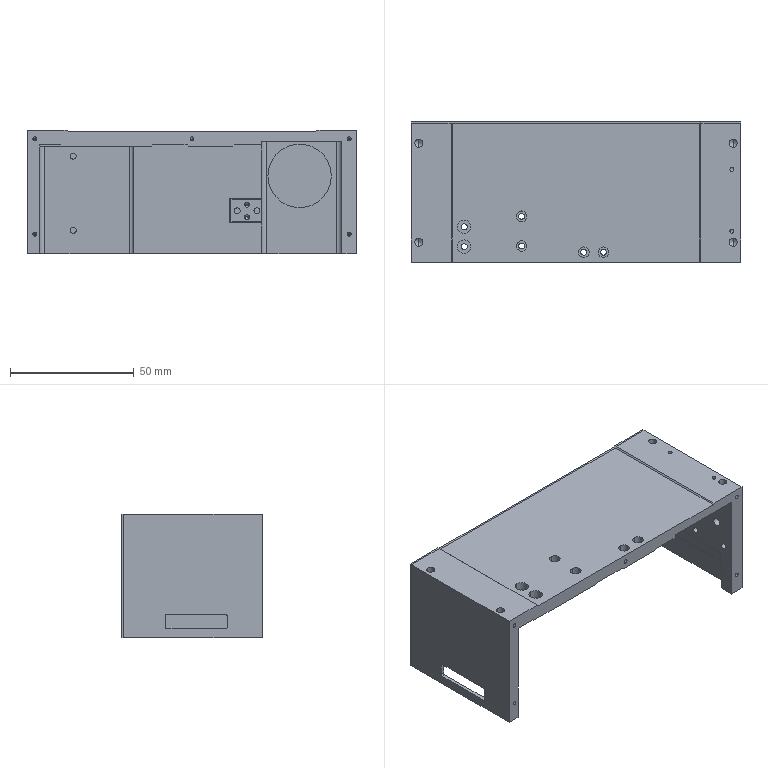NC program | NX | posted with a generic post | part box 133 x 56.74 x 50 mm
Lines 11184 to 11561 of 22463:
(11 , TOOL : D10JING)
N22336 T09 M6
N22338 G54
N22340 G17 G0 G90 X54.668 Y-35.392 B0. C0. S9500 M3
N22342 G43 Z30. H9
N22344 Z-10.4
N22346 G94 G1 Z-12.4 F1000.
N22348 X56.007 Y-34.61
N22350 G3 X56.502 Y-33.741 R1.
N22352 G1 X56.5 Y-33.295 F1200.
N22354 X56.499 Y-28.392
N22356 X56.5 Y-27.946
N22358 Y17.63
N22360 X26.5
N22362 G2 X23.5 Y16.63 R5.
N22364 G1 X-28.25
N22366 G2 X-32.833 Y19.63 R5.
N22368 G1 X-55.5
N22370 Y17.63
N22372 G2 X-59.5 Y12.731 R5.
N22374 G1 Y-17.471
N22376 G2 X-55.5 Y-22.37 R5.
N22378 G1 Y-27.946
N22380 X-55.501 Y-33.295
N22382 X-55.502 Y-33.741
N22384 G3 X-55.005 Y-34.609 R1.
N22386 G1 X-53.667 Y-35.388
N22388 Z-10.4
N22390 G0 Z30.
(111 , TOOL : D10JING)
N22392 X54.671 Y-35.397
N22394 Z-6.6
N22396 G1 Z-8.6 F1000.
N22398 X56.01 Y-34.611
N22400 G3 X56.503 Y-33.741 R1.
N22402 G1 X56.5 Y-33.295 F1200.
N22404 Y-27.946
N22406 Y17.63
N22408 X26.5
N22410 G2 X23.5 Y16.63 R5.
N22412 G1 X-10.429
N22414 G2 X-12.478 Y16.132 R4.981
N22416 G1 X-15.629 Y16.131
N22418 X-15.765 Y16.13
N22420 X-27.524
N22422 G2 X-30.33 Y16.989 R5.076
N22424 X-30.711 Y17.278 R3.745
N22426 X-32.833 Y19.63 R5.
N22428 G1 X-55.5
N22430 Y-27.946
N22432 X-55.501 Y-28.838
N22434 Y-33.295
N22436 X-55.503 Y-33.741
N22438 G3 X-55.006 Y-34.609 R1.
N22440 G1 X-53.668 Y-35.388
N22442 Z-6.6
N22444 G0 Z30.
N22446 X54.671 Y-35.397
N22448 Z-15.2
N22450 G1 Z-17.2 F1000.
N22452 X56.01 Y-34.611
N22454 G3 X56.503 Y-33.741 R1.
N22456 G1 X56.5 Y-33.295 F1200.
N22458 Y-27.946
N22460 Y17.63
N22462 X26.5
N22464 G2 X23.5 Y16.63 R5.
N22466 G1 X-2.939
N22468 G2 X-5.12 Y16.131 R5.
N22470 G1 X-15.738 Y16.13
N22472 X-28.25
N22474 G2 X-33.02 Y19.63 R5.
N22476 G1 X-55.5
N22478 Y-27.946
N22480 X-55.502 Y-33.741
N22482 G3 X-55.003 Y-34.607 R1.
N22484 G1 X-53.666 Y-35.38
N22486 Z-15.2
N22488 G0 Z30.
N22490 X54.67 Y-35.398
N22492 Z-23.8
N22494 G1 Z-25.8 F1000.
N22496 X56.01 Y-34.611
N22498 G3 X56.503 Y-33.741 R1.
N22500 G1 X56.5 Y-33.295 F1200.
N22502 Y-27.946
N22504 Y17.63
N22506 X26.5
N22508 G2 X23.5 Y16.63 R5.
N22510 G1 X-2.939
N22512 G2 X-5.12 Y16.13 R4.989
N22514 G1 X-15.765
N22516 X-28.25
N22518 G2 X-33.02 Y19.63 R5.
N22520 G1 X-55.5
N22522 Y-27.946
N22524 X-55.502 Y-33.741
N22526 G3 X-55.002 Y-34.607 R1.
N22528 G1 X-53.665 Y-35.38
N22530 Z-23.8
N22532 G0 Z30.
N22534 X54.67 Y-35.398
N22536 Z-32.4
N22538 G1 Z-34.4 F1000.
N22540 X56.009 Y-34.611
N22542 G3 X56.503 Y-33.741 R1.
N22544 G1 X56.499 Y-33.295 F1200.
N22546 X56.498 Y-28.392
N22548 X56.5 Y-27.946
N22550 Y17.63
N22552 X26.5
N22554 G2 X23.5 Y16.63 R5.
N22556 G1 X-2.938
N22558 G2 X-5.12 Y16.13 R4.981
N22560 G1 X-15.738
N22562 X-28.25
N22564 G2 X-33.02 Y19.63 R5.
N22566 G1 X-55.5
N22568 Y-27.946
N22570 Y-33.295
N22572 X-55.501 Y-33.741
N22574 G3 X-55.003 Y-34.608 R1.
N22576 G1 X-53.666 Y-35.384
N22578 Z-32.4
N22580 G0 Z30.
N22582 X54.67 Y-35.398
N22584 Z-41.
N22586 G1 Z-43. F1000.
N22588 X56.009 Y-34.611
N22590 G3 X56.502 Y-33.741 R1.
N22592 G1 X56.499 Y-33.295 F1200.
N22594 X56.5 Y-27.946
N22596 Y17.63
N22598 X26.5
N22600 G2 X23.5 Y16.63 R5.
N22602 G1 X-2.938
N22604 G2 X-5.12 Y16.13 R4.972
N22606 G1 X-15.765
N22608 X-23.249
N22610 G3 X-22.749 Y15.264 R1.
N22612 G1 X-20.785 Y14.13
N22614 Z-41.
N22616 G0 Z30.
N22618 X-35.063 Y2.523
N22620 Z-41.
N22622 G1 Z-43. F1000.
N22624 X-33.749 Y3.282
N22626 G3 X-33.249 Y4.148 R1.
N22628 G1 Y8.605 F1200.
N22630 Y9.942
N22632 X-33.25 Y11.349
N22634 Y19.63
N22636 X-55.5
N22638 Y-27.946
N22640 Y-33.295
N22642 X-55.501 Y-33.741
N22644 G3 X-55.002 Y-34.608 R1.
N22646 G1 X-53.665 Y-35.382
N22648 Z-41.
N22650 G0 Z30.
(FLOOR_WALL_2 , TOOL : D10JING)
N22652 X53.5 Y-12.87
N22654 Z-6.5
N22656 G1 Z-9.5 F1250.
N22658 X56.503
N22660 Y14.13
N22662 X59.5
N22664 Y-12.87
N22666 X53.5
N22668 Z-6.5
N22670 G0 Z30.
N22672 Y-13.37
N22674 Z-6.5
N22676 G1 Z-9.5
N22678 X56.5
N22680 X60.
N22682 Y14.63
N22684 X56.5
N22686 X53.5
N22688 Z-6.5
N22690 G0 Z30.
N22692 Y4.63
N22694 Z-40.5
N22696 G1 Z-43.5
N22698 X56. Y7.63
N22700 X25.49
N22702 G2 X18.871 Y12.38 R7.
N22704 G1 X56.
N22706 Y17.13
N22708 X26.662
N22710 Z-40.5
N22712 G0 Z30.
N22714 X53.5 Y4.63
N22716 Z-40.5
N22718 G1 Z-43.5
N22720 X56.5
N22722 Y7.63
N22724 Y17.63
N22726 X26.5
N22728 G2 X23.5 Y16.63 R5.
N22730 G1 X18.53
N22732 X15.53
N22734 Y13.63
N22736 Z-40.5
N22738 G0 Z30.
N22740 X11.5 Y-36.37
N22742 Z-40.5
N22744 G1 Z-43.5
N22746 Y-33.37
N22748 Y0.63
N22750 X16.125
N22752 Y-33.37
N22754 X20.75
N22756 Y0.63
N22758 X25.375
N22760 Y-33.37
N22762 X30.
N22764 Y0.63
N22766 X34.625
N22768 Y-33.37
N22770 X39.25
N22772 Y0.63
N22774 X43.875
N22776 Y-33.37
N22778 X48.5
N22780 Y0.63
N22782 Y3.63
N22784 Z-40.5
N22786 G0 Z30.
N22788 X56.5 Y-36.37
N22790 Z-40.5
N22792 G1 Z-43.5
N22794 Y-33.37
N22796 Y0.63
N22798 Y3.63
N22800 X53.5
N22802 Z-40.5
N22804 G0 Z30.
N22806 X10.5 Y-36.37
N22808 Z-41.
N22810 G1 Z-44.
N22812 Y-33.37
N22814 X7.5
N22816 Y-28.42
N22818 X10.5
N22820 Y-23.47
N22822 X7.5
N22824 Y-18.52
N22826 X10.5
N22828 Y-13.57
N22830 X7.5
N22832 Z-41.
N22834 G0 Z30.
N22836 X-22.5 Y-36.37
N22838 Z-41.
N22840 G1 Z-44.
N22842 Y-33.37
N22844 X-33.25
N22846 Y-28.42
N22848 X-22.5
N22850 Y-23.47
N22852 X-33.25
N22854 Y-18.52
N22856 X-22.5
N22858 Y-13.57
N22860 X-33.229
N22862 G2 X-32.104 Y-8.62 R15.
N22864 G1 X10.5
N22866 Y-3.67
N22868 X-28.762
N22870 X-30.711 Y1.28
N22872 X56.
N22874 Y6.23
N22876 X-32.86
N22878 G2 X-33.25 Y9.63 R15.
N22880 G1 Y11.18
N22882 X18.841
N22884 G2 X18. Y14.63 R7.5
N22886 G1 Y16.13
N22888 X-12.972
N22890 Z-41.
N22892 G0 Z30.
N22894 X-22. Y-36.37
N22896 Z-41.
N22898 G1 Z-44.
N22900 Y-33.37
N22902 Y-11.87
N22904 X7.
N22906 Y-33.37
N22908 Y-36.37
N22910 X11.
N22912 Y-33.37
N22914 Y0.63
N22916 X56.5
N22918 Y7.63
N22920 X25.5
N22922 G2 X18.5 Y14.63 R7.
N22924 G1 Y16.63
N22926 X-13.179
N22928 X-13.679 Y16.13
N22930 X-33.25
N22932 X-36.25
N22934 Z-41.
N22936 G0 Z30.
N22938 X-24.5 Y-12.37
N22940 Z-40.5
N22942 G1 Z-43.5
N22944 X-21.5
N22946 X6.5
N22948 Y-16.37
N22950 X-21.5
N22952 Y-20.37
N22954 X6.5
N22956 Y-24.37
N22958 X-21.5
N22960 X-24.5
N22962 Z-40.5
N22964 G0 Z30.
N22966 X-54.997 Y-36.37
N22968 Z-42.5
N22970 G1 Z-45.5
N22972 Y-33.37
N22974 Y19.13
N22976 X-50.508
N22978 Y-33.37
N22980 X-46.018
N22982 Y19.13
N22984 X-41.529
N22986 Y-33.37
N22988 X-37.039
N22990 Y19.13
N22992 X-33.75
N22994 Y9.63
N22996 G3 X-32.55 Y3.65 R15.5
N22998 G1 Y-8.39
N23000 G2 X-28.061 Y-2.37 R15.5
N23002 G1 Z-42.5
N23004 G0 Z30.
N23006 X-33.25 Y-36.37
N23008 Z-42.5
N23010 G1 Z-45.5
N23012 Y-33.37
N23014 Y-14.37
N23016 G2 X-27.25 Y-2.37 R15.
N23018 X-33.25 Y9.63 R15.
N23020 G1 Y19.63
N23022 X-55.5
N23024 Y-33.37
N23026 Y-36.37
N23028 Z-42.5
N23030 G0 Z30.
N23032 X-52.5 Y12.13
N23034 Z-10.
N23036 G1 Z-13.
N23038 X-55.503
N23040 Y-16.87
N23042 X-59.
N23044 Y12.13
N23046 X-52.5
N23048 Z-10.
N23050 G0 Z30.
N23052 Y12.63
N23054 Z-10.
N23056 G1 Z-13.
N23058 X-55.5
N23060 X-59.5
N23062 Y-17.37
N23064 X-55.5
N23066 X-52.5
N23068 Z-10.
N23070 G0 Z30.
N23072 M5